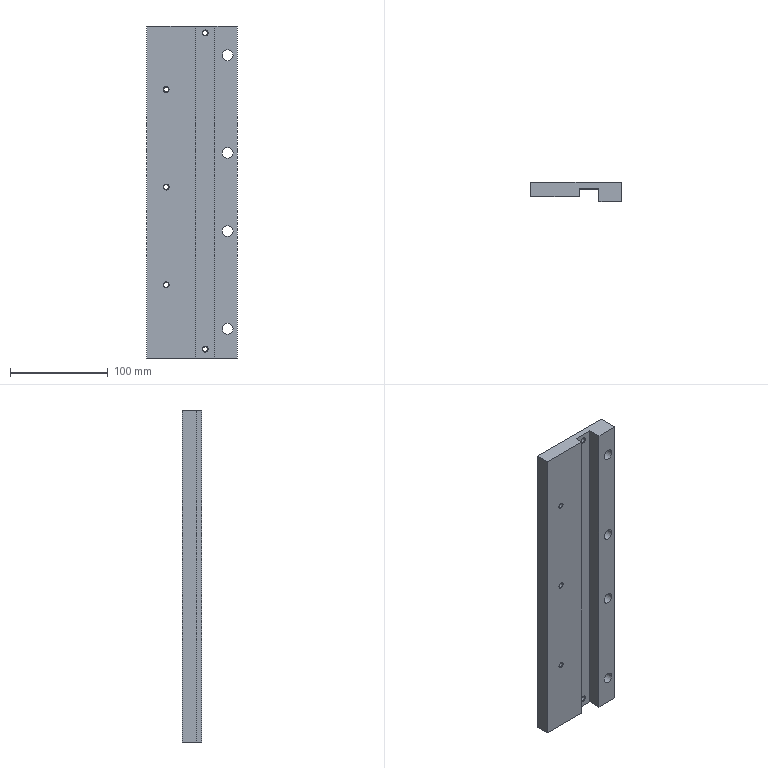Part | STEP file | 1 solid | 38 faces | box 92.98 x 19.5 x 340 mm | volume 434524 mm3 | cylinder 18 | cone 10 | plane 10 | commonest cylinder face diameters 5 x10 11 x8